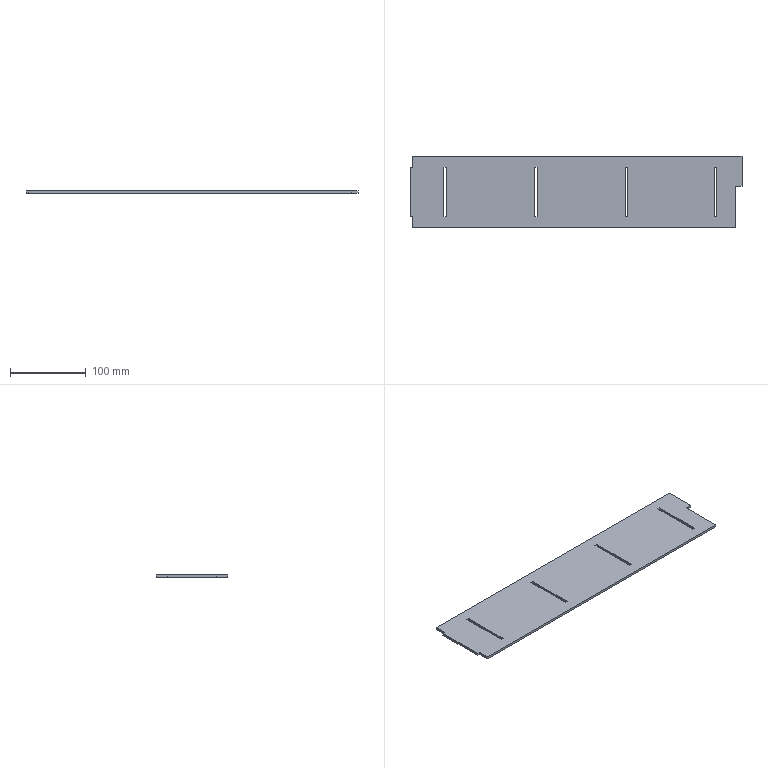Part | SolidWorks | features FlatPattern 1, SMBaseFlange 1, SheetMetal 1 | 1 solid | 28 faces | box 439 x 95 x 3.2 mm | volume 129037 mm3 | plane 28
STEP:
#1=CARTESIAN_POINT('',(218.,0.,3.2));
#2=VERTEX_POINT('',#1);
#3=CARTESIAN_POINT('',(-218.,0.,3.2));
#4=VERTEX_POINT('',#3);
#5=CARTESIAN_POINT('',(218.,0.,3.2));
#6=DIRECTION('',(-1.,0.,0.));
#7=VECTOR('',#6,1000.);
#8=LINE('',#5,#7);
#9=EDGE_CURVE('',#2,#4,#8,.T.);
#10=ORIENTED_EDGE('',*,*,#9,.T.);
#11=CARTESIAN_POINT('',(-218.,-15.,3.2));
#12=VERTEX_POINT('',#11);
#13=CARTESIAN_POINT('',(-218.,0.,3.2));
#14=DIRECTION('',(0.,-1.,0.));
#15=VECTOR('',#14,1000.);
#16=LINE('',#13,#15);
#17=EDGE_CURVE('',#4,#12,#16,.T.);
#18=ORIENTED_EDGE('',*,*,#17,.T.);
#19=CARTESIAN_POINT('',(-221.,-15.,3.2));
#20=VERTEX_POINT('',#19);
#21=CARTESIAN_POINT('',(-218.,-15.,3.2));
#22=DIRECTION('',(-1.,0.,0.));
#23=VECTOR('',#22,1000.);
#24=LINE('',#21,#23);
#25=EDGE_CURVE('',#12,#20,#24,.T.);
#26=ORIENTED_EDGE('',*,*,#25,.T.);
#27=CARTESIAN_POINT('',(-221.,-80.,3.2));
#28=VERTEX_POINT('',#27);
#29=CARTESIAN_POINT('',(-221.,-15.,3.2));
#30=DIRECTION('',(0.,-1.,0.));
#31=VECTOR('',#30,1000.);
#32=LINE('',#29,#31);
#33=EDGE_CURVE('',#20,#28,#32,.T.);
#34=ORIENTED_EDGE('',*,*,#33,.T.);
#35=CARTESIAN_POINT('',(-218.,-80.,3.2));
#36=VERTEX_POINT('',#35);
#37=CARTESIAN_POINT('',(-221.,-80.,3.2));
#38=DIRECTION('',(1.,0.,0.));
#39=VECTOR('',#38,1000.);
#40=LINE('',#37,#39);
#41=EDGE_CURVE('',#28,#36,#40,.T.);
#42=ORIENTED_EDGE('',*,*,#41,.T.);
#43=CARTESIAN_POINT('',(-218.,-95.,3.2));
#44=VERTEX_POINT('',#43);
#45=CARTESIAN_POINT('',(-218.,-80.,3.2));
#46=DIRECTION('',(0.,-1.,0.));
#47=VECTOR('',#46,1000.);
#48=LINE('',#45,#47);
#49=EDGE_CURVE('',#36,#44,#48,.T.);
#50=ORIENTED_EDGE('',*,*,#49,.T.);
#51=CARTESIAN_POINT('',(209.7,-95.,3.2));
#52=VERTEX_POINT('',#51);
#53=CARTESIAN_POINT('',(-218.,-95.,3.2));
#54=DIRECTION('',(1.,0.,0.));
#55=VECTOR('',#54,1000.);
#56=LINE('',#53,#55);
#57=EDGE_CURVE('',#44,#52,#56,.T.);
#58=ORIENTED_EDGE('',*,*,#57,.T.);
#59=CARTESIAN_POINT('',(209.7,-39.7,3.2));
#60=VERTEX_POINT('',#59);
#61=CARTESIAN_POINT('',(209.7,-95.,3.2));
#62=DIRECTION('',(0.,1.,0.));
#63=VECTOR('',#62,1000.);
#64=LINE('',#61,#63);
#65=EDGE_CURVE('',#52,#60,#64,.T.);
#66=ORIENTED_EDGE('',*,*,#65,.T.);
#67=CARTESIAN_POINT('',(218.,-39.7,3.2));
#68=VERTEX_POINT('',#67);
#69=CARTESIAN_POINT('',(209.7,-39.7,3.2));
#70=DIRECTION('',(1.,0.,0.));
#71=VECTOR('',#70,1000.);
#72=LINE('',#69,#71);
#73=EDGE_CURVE('',#60,#68,#72,.T.);
#74=ORIENTED_EDGE('',*,*,#73,.T.);
#75=CARTESIAN_POINT('',(218.,-39.7,3.2));
#76=DIRECTION('',(0.,1.,0.));
#77=VECTOR('',#76,1000.);
#78=LINE('',#75,#77);
#79=EDGE_CURVE('',#68,#2,#78,.T.);
#80=ORIENTED_EDGE('',*,*,#79,.T.);
#81=EDGE_LOOP('',(#10,#18,#26,#34,#42,#50,#58,#66,#74,#80));
#82=FACE_OUTER_BOUND('',#81,.T.);
#83=CARTESIAN_POINT('',(181.5,-80.,3.2));
#84=VERTEX_POINT('',#83);
#85=CARTESIAN_POINT('',(184.7,-80.,3.2));
#86=VERTEX_POINT('',#85);
#87=CARTESIAN_POINT('',(181.5,-80.,3.2));
#88=DIRECTION('',(1.,0.,0.));
#89=VECTOR('',#88,1000.);
#90=LINE('',#87,#89);
#91=EDGE_CURVE('',#84,#86,#90,.T.);
#92=ORIENTED_EDGE('',*,*,#91,.F.);
#93=CARTESIAN_POINT('',(181.5,-15.,3.2));
#94=VERTEX_POINT('',#93);
#95=CARTESIAN_POINT('',(181.5,-15.,3.2));
#96=DIRECTION('',(0.,-1.,0.));
#97=VECTOR('',#96,1000.);
#98=LINE('',#95,#97);
#99=EDGE_CURVE('',#94,#84,#98,.T.);
#100=ORIENTED_EDGE('',*,*,#99,.F.);
#101=CARTESIAN_POINT('',(184.7,-15.,3.2));
#102=VERTEX_POINT('',#101);
#103=CARTESIAN_POINT('',(181.5,-15.,3.2));
#104=DIRECTION('',(-1.,0.,0.));
#105=VECTOR('',#104,1000.);
#106=LINE('',#103,#105);
#107=EDGE_CURVE('',#102,#94,#106,.T.);
#108=ORIENTED_EDGE('',*,*,#107,.F.);
#109=CARTESIAN_POINT('',(184.7,-15.,3.2));
#110=DIRECTION('',(0.,1.,0.));
#111=VECTOR('',#110,1000.);
#112=LINE('',#109,#111);
#113=EDGE_CURVE('',#86,#102,#112,.T.);
#114=ORIENTED_EDGE('',*,*,#113,.F.);
#115=EDGE_LOOP('',(#92,#100,#108,#114));
#116=FACE_BOUND('',#115,.T.);
#117=CARTESIAN_POINT('',(63.8,-80.,3.2));
#118=VERTEX_POINT('',#117);
#119=CARTESIAN_POINT('',(67.,-80.,3.2));
#120=VERTEX_POINT('',#119);
#121=CARTESIAN_POINT('',(63.8,-80.,3.2));
#122=DIRECTION('',(1.,0.,0.));
#123=VECTOR('',#122,1000.);
#124=LINE('',#121,#123);
#125=EDGE_CURVE('',#118,#120,#124,.T.);
#126=ORIENTED_EDGE('',*,*,#125,.F.);
#127=CARTESIAN_POINT('',(63.8,-15.,3.2));
#128=VERTEX_POINT('',#127);
#129=CARTESIAN_POINT('',(63.8,-15.,3.2));
#130=DIRECTION('',(0.,-1.,0.));
#131=VECTOR('',#130,1000.);
#132=LINE('',#129,#131);
#133=EDGE_CURVE('',#128,#118,#132,.T.);
#134=ORIENTED_EDGE('',*,*,#133,.F.);
#135=CARTESIAN_POINT('',(67.,-15.,3.2));
#136=VERTEX_POINT('',#135);
#137=CARTESIAN_POINT('',(63.8,-15.,3.2));
#138=DIRECTION('',(-1.,0.,0.));
#139=VECTOR('',#138,1000.);
#140=LINE('',#137,#139);
#141=EDGE_CURVE('',#136,#128,#140,.T.);
#142=ORIENTED_EDGE('',*,*,#141,.F.);
#143=CARTESIAN_POINT('',(67.,-15.,3.2));
#144=DIRECTION('',(0.,1.,0.));
#145=VECTOR('',#144,1000.);
#146=LINE('',#143,#145);
#147=EDGE_CURVE('',#120,#136,#146,.T.);
#148=ORIENTED_EDGE('',*,*,#147,.F.);
#149=EDGE_LOOP('',(#126,#134,#142,#148));
#150=FACE_BOUND('',#149,.T.);
#151=CARTESIAN_POINT('',(-56.2,-80.,3.2));
#152=VERTEX_POINT('',#151);
#153=CARTESIAN_POINT('',(-53.,-80.,3.2));
#154=VERTEX_POINT('',#153);
#155=CARTESIAN_POINT('',(-56.2,-80.,3.2));
#156=DIRECTION('',(1.,0.,0.));
#157=VECTOR('',#156,1000.);
#158=LINE('',#155,#157);
#159=EDGE_CURVE('',#152,#154,#158,.T.);
#160=ORIENTED_EDGE('',*,*,#159,.F.);
#161=CARTESIAN_POINT('',(-56.2,-15.,3.2));
#162=VERTEX_POINT('',#161);
#163=CARTESIAN_POINT('',(-56.2,-15.,3.2));
#164=DIRECTION('',(0.,-1.,0.));
#165=VECTOR('',#164,1000.);
#166=LINE('',#163,#165);
#167=EDGE_CURVE('',#162,#152,#166,.T.);
#168=ORIENTED_EDGE('',*,*,#167,.F.);
#169=CARTESIAN_POINT('',(-53.,-15.,3.2));
#170=VERTEX_POINT('',#169);
#171=CARTESIAN_POINT('',(-56.2,-15.,3.2));
#172=DIRECTION('',(-1.,0.,0.));
#173=VECTOR('',#172,1000.);
#174=LINE('',#171,#173);
#175=EDGE_CURVE('',#170,#162,#174,.T.);
#176=ORIENTED_EDGE('',*,*,#175,.F.);
#177=CARTESIAN_POINT('',(-53.,-15.,3.2));
#178=DIRECTION('',(0.,1.,0.));
#179=VECTOR('',#178,1000.);
#180=LINE('',#177,#179);
#181=EDGE_CURVE('',#154,#170,#180,.T.);
#182=ORIENTED_EDGE('',*,*,#181,.F.);
#183=EDGE_LOOP('',(#160,#168,#176,#182));
#184=FACE_BOUND('',#183,.T.);
#185=CARTESIAN_POINT('',(-176.2,-80.,3.2));
#186=VERTEX_POINT('',#185);
#187=CARTESIAN_POINT('',(-173.,-80.,3.2));
#188=VERTEX_POINT('',#187);
#189=CARTESIAN_POINT('',(-176.2,-80.,3.2));
#190=DIRECTION('',(1.,0.,0.));
#191=VECTOR('',#190,1000.);
#192=LINE('',#189,#191);
#193=EDGE_CURVE('',#186,#188,#192,.T.);
#194=ORIENTED_EDGE('',*,*,#193,.F.);
#195=CARTESIAN_POINT('',(-176.2,-15.,3.2));
#196=VERTEX_POINT('',#195);
#197=CARTESIAN_POINT('',(-176.2,-15.,3.2));
#198=DIRECTION('',(0.,-1.,0.));
#199=VECTOR('',#198,1000.);
#200=LINE('',#197,#199);
#201=EDGE_CURVE('',#196,#186,#200,.T.);
#202=ORIENTED_EDGE('',*,*,#201,.F.);
#203=CARTESIAN_POINT('',(-173.,-15.,3.2));
#204=VERTEX_POINT('',#203);
#205=CARTESIAN_POINT('',(-176.2,-15.,3.2));
#206=DIRECTION('',(-1.,0.,0.));
#207=VECTOR('',#206,1000.);
#208=LINE('',#205,#207);
#209=EDGE_CURVE('',#204,#196,#208,.T.);
#210=ORIENTED_EDGE('',*,*,#209,.F.);
#211=CARTESIAN_POINT('',(-173.,-15.,3.2));
#212=DIRECTION('',(0.,1.,0.));
#213=VECTOR('',#212,1000.);
#214=LINE('',#211,#213);
#215=EDGE_CURVE('',#188,#204,#214,.T.);
#216=ORIENTED_EDGE('',*,*,#215,.F.);
#217=EDGE_LOOP('',(#194,#202,#210,#216));
#218=FACE_BOUND('',#217,.T.);
#219=CARTESIAN_POINT('',(0.,0.,3.2));
#220=DIRECTION('',(0.,0.,1.));
#221=DIRECTION('',(1.,0.,0.));
#222=AXIS2_PLACEMENT_3D('',#219,#220,#221);
#223=PLANE('',#222);
#224=ADVANCED_FACE('',(#82,#116,#150,#184,#218),#223,.T.);
#225=CARTESIAN_POINT('',(-56.2,-15.,0.));
#226=VERTEX_POINT('',#225);
#227=CARTESIAN_POINT('',(-56.2,-80.,0.));
#228=VERTEX_POINT('',#227);
#229=CARTESIAN_POINT('',(-56.2,-15.,0.));
#230=DIRECTION('',(0.,-1.,0.));
#231=VECTOR('',#230,1000.);
#232=LINE('',#229,#231);
#233=EDGE_CURVE('',#226,#228,#232,.T.);
#234=ORIENTED_EDGE('',*,*,#233,.T.);
#235=CARTESIAN_POINT('',(-53.,-80.,0.));
#236=VERTEX_POINT('',#235);
#237=CARTESIAN_POINT('',(-56.2,-80.,0.));
#238=DIRECTION('',(1.,0.,0.));
#239=VECTOR('',#238,1000.);
#240=LINE('',#237,#239);
#241=EDGE_CURVE('',#228,#236,#240,.T.);
#242=ORIENTED_EDGE('',*,*,#241,.T.);
#243=CARTESIAN_POINT('',(-53.,-15.,0.));
#244=VERTEX_POINT('',#243);
#245=CARTESIAN_POINT('',(-53.,-15.,0.));
#246=DIRECTION('',(0.,1.,0.));
#247=VECTOR('',#246,1000.);
#248=LINE('',#245,#247);
#249=EDGE_CURVE('',#236,#244,#248,.T.);
#250=ORIENTED_EDGE('',*,*,#249,.T.);
#251=CARTESIAN_POINT('',(-56.2,-15.,0.));
#252=DIRECTION('',(-1.,0.,0.));
#253=VECTOR('',#252,1000.);
#254=LINE('',#251,#253);
#255=EDGE_CURVE('',#244,#226,#254,.T.);
#256=ORIENTED_EDGE('',*,*,#255,.T.);
#257=EDGE_LOOP('',(#234,#242,#250,#256));
#258=FACE_BOUND('',#257,.T.);
#259=CARTESIAN_POINT('',(181.5,-15.,0.));
#260=VERTEX_POINT('',#259);
#261=CARTESIAN_POINT('',(181.5,-80.,0.));
#262=VERTEX_POINT('',#261);
#263=CARTESIAN_POINT('',(181.5,-15.,0.));
#264=DIRECTION('',(0.,-1.,0.));
#265=VECTOR('',#264,1000.);
#266=LINE('',#263,#265);
#267=EDGE_CURVE('',#260,#262,#266,.T.);
#268=ORIENTED_EDGE('',*,*,#267,.T.);
#269=CARTESIAN_POINT('',(184.7,-80.,0.));
#270=VERTEX_POINT('',#269);
#271=CARTESIAN_POINT('',(181.5,-80.,0.));
#272=DIRECTION('',(1.,0.,0.));
#273=VECTOR('',#272,1000.);
#274=LINE('',#271,#273);
#275=EDGE_CURVE('',#262,#270,#274,.T.);
#276=ORIENTED_EDGE('',*,*,#275,.T.);
#277=CARTESIAN_POINT('',(184.7,-15.,0.));
#278=VERTEX_POINT('',#277);
#279=CARTESIAN_POINT('',(184.7,-15.,0.));
#280=DIRECTION('',(0.,1.,0.));
#281=VECTOR('',#280,1000.);
#282=LINE('',#279,#281);
#283=EDGE_CURVE('',#270,#278,#282,.T.);
#284=ORIENTED_EDGE('',*,*,#283,.T.);
#285=CARTESIAN_POINT('',(181.5,-15.,0.));
#286=DIRECTION('',(-1.,0.,0.));
#287=VECTOR('',#286,1000.);
#288=LINE('',#285,#287);
#289=EDGE_CURVE('',#278,#260,#288,.T.);
#290=ORIENTED_EDGE('',*,*,#289,.T.);
#291=EDGE_LOOP('',(#268,#276,#284,#290));
#292=FACE_BOUND('',#291,.T.);
#293=CARTESIAN_POINT('',(218.,0.,0.));
#294=VERTEX_POINT('',#293);
#295=CARTESIAN_POINT('',(-218.,0.,0.));
#296=VERTEX_POINT('',#295);
#297=CARTESIAN_POINT('',(218.,0.,0.));
#298=DIRECTION('',(-1.,0.,0.));
#299=VECTOR('',#298,1000.);
#300=LINE('',#297,#299);
#301=EDGE_CURVE('',#294,#296,#300,.T.);
#302=ORIENTED_EDGE('',*,*,#301,.F.);
#303=CARTESIAN_POINT('',(218.,-39.7,0.));
#304=VERTEX_POINT('',#303);
#305=CARTESIAN_POINT('',(218.,-39.7,0.));
#306=DIRECTION('',(0.,1.,0.));
#307=VECTOR('',#306,1000.);
#308=LINE('',#305,#307);
#309=EDGE_CURVE('',#304,#294,#308,.T.);
#310=ORIENTED_EDGE('',*,*,#309,.F.);
#311=CARTESIAN_POINT('',(209.7,-39.7,0.));
#312=VERTEX_POINT('',#311);
#313=CARTESIAN_POINT('',(209.7,-39.7,0.));
#314=DIRECTION('',(1.,0.,0.));
#315=VECTOR('',#314,1000.);
#316=LINE('',#313,#315);
#317=EDGE_CURVE('',#312,#304,#316,.T.);
#318=ORIENTED_EDGE('',*,*,#317,.F.);
#319=CARTESIAN_POINT('',(209.7,-95.,0.));
#320=VERTEX_POINT('',#319);
#321=CARTESIAN_POINT('',(209.7,-95.,0.));
#322=DIRECTION('',(0.,1.,0.));
#323=VECTOR('',#322,1000.);
#324=LINE('',#321,#323);
#325=EDGE_CURVE('',#320,#312,#324,.T.);
#326=ORIENTED_EDGE('',*,*,#325,.F.);
#327=CARTESIAN_POINT('',(-218.,-95.,0.));
#328=VERTEX_POINT('',#327);
#329=CARTESIAN_POINT('',(-218.,-95.,0.));
#330=DIRECTION('',(1.,0.,0.));
#331=VECTOR('',#330,1000.);
#332=LINE('',#329,#331);
#333=EDGE_CURVE('',#328,#320,#332,.T.);
#334=ORIENTED_EDGE('',*,*,#333,.F.);
#335=CARTESIAN_POINT('',(-218.,-80.,0.));
#336=VERTEX_POINT('',#335);
#337=CARTESIAN_POINT('',(-218.,-80.,0.));
#338=DIRECTION('',(0.,-1.,0.));
#339=VECTOR('',#338,1000.);
#340=LINE('',#337,#339);
#341=EDGE_CURVE('',#336,#328,#340,.T.);
#342=ORIENTED_EDGE('',*,*,#341,.F.);
#343=CARTESIAN_POINT('',(-221.,-80.,0.));
#344=VERTEX_POINT('',#343);
#345=CARTESIAN_POINT('',(-221.,-80.,0.));
#346=DIRECTION('',(1.,0.,0.));
#347=VECTOR('',#346,1000.);
#348=LINE('',#345,#347);
#349=EDGE_CURVE('',#344,#336,#348,.T.);
#350=ORIENTED_EDGE('',*,*,#349,.F.);
#351=CARTESIAN_POINT('',(-221.,-15.,0.));
#352=VERTEX_POINT('',#351);
#353=CARTESIAN_POINT('',(-221.,-15.,0.));
#354=DIRECTION('',(0.,-1.,0.));
#355=VECTOR('',#354,1000.);
#356=LINE('',#353,#355);
#357=EDGE_CURVE('',#352,#344,#356,.T.);
#358=ORIENTED_EDGE('',*,*,#357,.F.);
#359=CARTESIAN_POINT('',(-218.,-15.,0.));
#360=VERTEX_POINT('',#359);
#361=CARTESIAN_POINT('',(-218.,-15.,0.));
#362=DIRECTION('',(-1.,0.,0.));
#363=VECTOR('',#362,1000.);
#364=LINE('',#361,#363);
#365=EDGE_CURVE('',#360,#352,#364,.T.);
#366=ORIENTED_EDGE('',*,*,#365,.F.);
#367=CARTESIAN_POINT('',(-218.,0.,0.));
#368=DIRECTION('',(0.,-1.,0.));
#369=VECTOR('',#368,1000.);
#370=LINE('',#367,#369);
#371=EDGE_CURVE('',#296,#360,#370,.T.);
#372=ORIENTED_EDGE('',*,*,#371,.F.);
#373=EDGE_LOOP('',(#302,#310,#318,#326,#334,#342,#350,#358,#366,#372));
#374=FACE_OUTER_BOUND('',#373,.T.);
#375=CARTESIAN_POINT('',(63.8,-15.,0.));
#376=VERTEX_POINT('',#375);
#377=CARTESIAN_POINT('',(63.8,-80.,0.));
#378=VERTEX_POINT('',#377);
#379=CARTESIAN_POINT('',(63.8,-15.,0.));
#380=DIRECTION('',(0.,-1.,0.));
#381=VECTOR('',#380,1000.);
#382=LINE('',#379,#381);
#383=EDGE_CURVE('',#376,#378,#382,.T.);
#384=ORIENTED_EDGE('',*,*,#383,.T.);
#385=CARTESIAN_POINT('',(67.,-80.,0.));
#386=VERTEX_POINT('',#385);
#387=CARTESIAN_POINT('',(63.8,-80.,0.));
#388=DIRECTION('',(1.,0.,0.));
#389=VECTOR('',#388,1000.);
#390=LINE('',#387,#389);
#391=EDGE_CURVE('',#378,#386,#390,.T.);
#392=ORIENTED_EDGE('',*,*,#391,.T.);
#393=CARTESIAN_POINT('',(67.,-15.,0.));
#394=VERTEX_POINT('',#393);
#395=CARTESIAN_POINT('',(67.,-15.,0.));
#396=DIRECTION('',(0.,1.,0.));
#397=VECTOR('',#396,1000.);
#398=LINE('',#395,#397);
#399=EDGE_CURVE('',#386,#394,#398,.T.);
#400=ORIENTED_EDGE('',*,*,#399,.T.);
#401=CARTESIAN_POINT('',(63.8,-15.,0.));
#402=DIRECTION('',(-1.,0.,0.));
#403=VECTOR('',#402,1000.);
#404=LINE('',#401,#403);
#405=EDGE_CURVE('',#394,#376,#404,.T.);
#406=ORIENTED_EDGE('',*,*,#405,.T.);
#407=EDGE_LOOP('',(#384,#392,#400,#406));
#408=FACE_BOUND('',#407,.T.);
#409=CARTESIAN_POINT('',(-176.2,-15.,0.));
#410=VERTEX_POINT('',#409);
#411=CARTESIAN_POINT('',(-176.2,-80.,0.));
#412=VERTEX_POINT('',#411);
#413=CARTESIAN_POINT('',(-176.2,-15.,0.));
#414=DIRECTION('',(0.,-1.,0.));
#415=VECTOR('',#414,1000.);
#416=LINE('',#413,#415);
#417=EDGE_CURVE('',#410,#412,#416,.T.);
#418=ORIENTED_EDGE('',*,*,#417,.T.);
#419=CARTESIAN_POINT('',(-173.,-80.,0.));
#420=VERTEX_POINT('',#419);
#421=CARTESIAN_POINT('',(-176.2,-80.,0.));
#422=DIRECTION('',(1.,0.,0.));
#423=VECTOR('',#422,1000.);
#424=LINE('',#421,#423);
#425=EDGE_CURVE('',#412,#420,#424,.T.);
#426=ORIENTED_EDGE('',*,*,#425,.T.);
#427=CARTESIAN_POINT('',(-173.,-15.,0.));
#428=VERTEX_POINT('',#427);
#429=CARTESIAN_POINT('',(-173.,-15.,0.));
#430=DIRECTION('',(0.,1.,0.));
#431=VECTOR('',#430,1000.);
#432=LINE('',#429,#431);
#433=EDGE_CURVE('',#420,#428,#432,.T.);
#434=ORIENTED_EDGE('',*,*,#433,.T.);
#435=CARTESIAN_POINT('',(-176.2,-15.,0.));
#436=DIRECTION('',(-1.,0.,0.));
#437=VECTOR('',#436,1000.);
#438=LINE('',#435,#437);
#439=EDGE_CURVE('',#428,#410,#438,.T.);
#440=ORIENTED_EDGE('',*,*,#439,.T.);
#441=EDGE_LOOP('',(#418,#426,#434,#440));
#442=FACE_BOUND('',#441,.T.);
#443=CARTESIAN_POINT('',(0.,0.,0.));
#444=DIRECTION('',(0.,0.,1.));
#445=DIRECTION('',(1.,0.,0.));
#446=AXIS2_PLACEMENT_3D('',#443,#444,#445);
#447=PLANE('',#446);
#448=ADVANCED_FACE('',(#258,#292,#374,#408,#442),#447,.F.);
#449=ORIENTED_EDGE('',*,*,#301,.T.);
#450=CARTESIAN_POINT('',(-218.,0.,3.2));
#451=DIRECTION('',(0.,0.,-1.));
#452=VECTOR('',#451,1000.);
#453=LINE('',#450,#452);
#454=EDGE_CURVE('',#4,#296,#453,.T.);
#455=ORIENTED_EDGE('',*,*,#454,.F.);
#456=ORIENTED_EDGE('',*,*,#9,.F.);
#457=CARTESIAN_POINT('',(218.,0.,3.2));
#458=DIRECTION('',(0.,0.,-1.));
#459=VECTOR('',#458,1000.);
#460=LINE('',#457,#459);
#461=EDGE_CURVE('',#2,#294,#460,.T.);
#462=ORIENTED_EDGE('',*,*,#461,.T.);
#463=EDGE_LOOP('',(#449,#455,#456,#462));
#464=FACE_OUTER_BOUND('',#463,.T.);
#465=CARTESIAN_POINT('',(218.,0.,3.2));
#466=DIRECTION('',(0.,-1.,0.));
#467=DIRECTION('',(1.,0.,0.));
#468=AXIS2_PLACEMENT_3D('',#465,#466,#467);
#469=PLANE('',#468);
#470=ADVANCED_FACE('',(#464),#469,.F.);
#471=ORIENTED_EDGE('',*,*,#371,.T.);
#472=CARTESIAN_POINT('',(-218.,-15.,3.2));
#473=DIRECTION('',(0.,0.,-1.));
#474=VECTOR('',#473,1000.);
#475=LINE('',#472,#474);
#476=EDGE_CURVE('',#12,#360,#475,.T.);
#477=ORIENTED_EDGE('',*,*,#476,.F.);
#478=ORIENTED_EDGE('',*,*,#17,.F.);
#479=ORIENTED_EDGE('',*,*,#454,.T.);
#480=EDGE_LOOP('',(#471,#477,#478,#479));
#481=FACE_OUTER_BOUND('',#480,.T.);
#482=CARTESIAN_POINT('',(-218.,0.,3.2));
#483=DIRECTION('',(1.,0.,0.));
#484=DIRECTION('',(0.,0.,-1.));
#485=AXIS2_PLACEMENT_3D('',#482,#483,#484);
#486=PLANE('',#485);
#487=ADVANCED_FACE('',(#481),#486,.F.);
#488=ORIENTED_EDGE('',*,*,#365,.T.);
#489=CARTESIAN_POINT('',(-221.,-15.,3.2));
#490=DIRECTION('',(0.,0.,-1.));
#491=VECTOR('',#490,1000.);
#492=LINE('',#489,#491);
#493=EDGE_CURVE('',#20,#352,#492,.T.);
#494=ORIENTED_EDGE('',*,*,#493,.F.);
#495=ORIENTED_EDGE('',*,*,#25,.F.);
#496=ORIENTED_EDGE('',*,*,#476,.T.);
#497=EDGE_LOOP('',(#488,#494,#495,#496));
#498=FACE_OUTER_BOUND('',#497,.T.);
#499=CARTESIAN_POINT('',(-218.,-15.,3.2));
#500=DIRECTION('',(0.,-1.,0.));
#501=DIRECTION('',(0.,0.,-1.));
#502=AXIS2_PLACEMENT_3D('',#499,#500,#501);
#503=PLANE('',#502);
#504=ADVANCED_FACE('',(#498),#503,.F.);
#505=ORIENTED_EDGE('',*,*,#357,.T.);
#506=CARTESIAN_POINT('',(-221.,-80.,3.2));
#507=DIRECTION('',(0.,0.,-1.));
#508=VECTOR('',#507,1000.);
#509=LINE('',#506,#508);
#510=EDGE_CURVE('',#28,#344,#509,.T.);
#511=ORIENTED_EDGE('',*,*,#510,.F.);
#512=ORIENTED_EDGE('',*,*,#33,.F.);
#513=ORIENTED_EDGE('',*,*,#493,.T.);
#514=EDGE_LOOP('',(#505,#511,#512,#513));
#515=FACE_OUTER_BOUND('',#514,.T.);
#516=CARTESIAN_POINT('',(-221.,-15.,3.2));
#517=DIRECTION('',(1.,0.,0.));
#518=DIRECTION('',(0.,1.,0.));
#519=AXIS2_PLACEMENT_3D('',#516,#517,#518);
#520=PLANE('',#519);
#521=ADVANCED_FACE('',(#515),#520,.F.);
#522=ORIENTED_EDGE('',*,*,#349,.T.);
#523=CARTESIAN_POINT('',(-218.,-80.,3.2));
#524=DIRECTION('',(0.,0.,-1.));
#525=VECTOR('',#524,1000.);
#526=LINE('',#523,#525);
#527=EDGE_CURVE('',#36,#336,#526,.T.);
#528=ORIENTED_EDGE('',*,*,#527,.F.);
#529=ORIENTED_EDGE('',*,*,#41,.F.);
#530=ORIENTED_EDGE('',*,*,#510,.T.);
#531=EDGE_LOOP('',(#522,#528,#529,#530));
#532=FACE_OUTER_BOUND('',#531,.T.);
#533=CARTESIAN_POINT('',(-221.,-80.,3.2));
#534=DIRECTION('',(0.,1.,0.));
#535=DIRECTION('',(0.,0.,1.));
#536=AXIS2_PLACEMENT_3D('',#533,#534,#535);
#537=PLANE('',#536);
#538=ADVANCED_FACE('',(#532),#537,.F.);
#539=ORIENTED_EDGE('',*,*,#341,.T.);
#540=CARTESIAN_POINT('',(-218.,-95.,3.2));
#541=DIRECTION('',(0.,0.,-1.));
#542=VECTOR('',#541,1000.);
#543=LINE('',#540,#542);
#544=EDGE_CURVE('',#44,#328,#543,.T.);
#545=ORIENTED_EDGE('',*,*,#544,.F.);
#546=ORIENTED_EDGE('',*,*,#49,.F.);
#547=ORIENTED_EDGE('',*,*,#527,.T.);
#548=EDGE_LOOP('',(#539,#545,#546,#547));
#549=FACE_OUTER_BOUND('',#548,.T.);
#550=CARTESIAN_POINT('',(-218.,-80.,3.2));
#551=DIRECTION('',(1.,0.,0.));
#552=DIRECTION('',(0.,0.,-1.));
#553=AXIS2_PLACEMENT_3D('',#550,#551,#552);
#554=PLANE('',#553);
#555=ADVANCED_FACE('',(#549),#554,.F.);
#556=ORIENTED_EDGE('',*,*,#333,.T.);
#557=CARTESIAN_POINT('',(209.7,-95.,3.2));
#558=DIRECTION('',(0.,0.,-1.));
#559=VECTOR('',#558,1000.);
#560=LINE('',#557,#559);
#561=EDGE_CURVE('',#52,#320,#560,.T.);
#562=ORIENTED_EDGE('',*,*,#561,.F.);
#563=ORIENTED_EDGE('',*,*,#57,.F.);
#564=ORIENTED_EDGE('',*,*,#544,.T.);
#565=EDGE_LOOP('',(#556,#562,#563,#564));
#566=FACE_OUTER_BOUND('',#565,.T.);
#567=CARTESIAN_POINT('',(-218.,-95.,3.2));
#568=DIRECTION('',(0.,1.,0.));
#569=DIRECTION('',(0.,0.,1.));
#570=AXIS2_PLACEMENT_3D('',#567,#568,#569);
#571=PLANE('',#570);
#572=ADVANCED_FACE('',(#566),#571,.F.);
#573=ORIENTED_EDGE('',*,*,#325,.T.);
#574=CARTESIAN_POINT('',(209.7,-39.7,3.2));
#575=DIRECTION('',(0.,0.,-1.));
#576=VECTOR('',#575,1000.);
#577=LINE('',#574,#576);
#578=EDGE_CURVE('',#60,#312,#577,.T.);
#579=ORIENTED_EDGE('',*,*,#578,.F.);
#580=ORIENTED_EDGE('',*,*,#65,.F.);
#581=ORIENTED_EDGE('',*,*,#561,.T.);
#582=EDGE_LOOP('',(#573,#579,#580,#581));
#583=FACE_OUTER_BOUND('',#582,.T.);
#584=CARTESIAN_POINT('',(209.7,-95.,3.2));
#585=DIRECTION('',(-1.,0.,0.));
#586=DIRECTION('',(0.,0.,1.));
#587=AXIS2_PLACEMENT_3D('',#584,#585,#586);
#588=PLANE('',#587);
#589=ADVANCED_FACE('',(#583),#588,.F.);
#590=ORIENTED_EDGE('',*,*,#317,.T.);
#591=CARTESIAN_POINT('',(218.,-39.7,3.2));
#592=DIRECTION('',(0.,0.,-1.));
#593=VECTOR('',#592,1000.);
#594=LINE('',#591,#593);
#595=EDGE_CURVE('',#68,#304,#594,.T.);
#596=ORIENTED_EDGE('',*,*,#595,.F.);
#597=ORIENTED_EDGE('',*,*,#73,.F.);
#598=ORIENTED_EDGE('',*,*,#578,.T.);
#599=EDGE_LOOP('',(#590,#596,#597,#598));
#600=FACE_OUTER_BOUND('',#599,.T.);
#601=CARTESIAN_POINT('',(209.7,-39.7,3.2));
#602=DIRECTION('',(0.,1.,0.));
#603=DIRECTION('',(0.,0.,1.));
#604=AXIS2_PLACEMENT_3D('',#601,#602,#603);
#605=PLANE('',#604);
#606=ADVANCED_FACE('',(#600),#605,.F.);
#607=ORIENTED_EDGE('',*,*,#309,.T.);
#608=ORIENTED_EDGE('',*,*,#461,.F.);
#609=ORIENTED_EDGE('',*,*,#79,.F.);
#610=ORIENTED_EDGE('',*,*,#595,.T.);
#611=EDGE_LOOP('',(#607,#608,#609,#610));
#612=FACE_OUTER_BOUND('',#611,.T.);
#613=CARTESIAN_POINT('',(218.,-39.7,3.2));
#614=DIRECTION('',(-1.,0.,0.));
#615=DIRECTION('',(0.,0.,1.));
#616=AXIS2_PLACEMENT_3D('',#613,#614,#615);
#617=PLANE('',#616);
#618=ADVANCED_FACE('',(#612),#617,.F.);
#619=ORIENTED_EDGE('',*,*,#267,.F.);
#620=CARTESIAN_POINT('',(181.5,-15.,3.2));
#621=DIRECTION('',(0.,0.,-1.));
#622=VECTOR('',#621,1000.);
#623=LINE('',#620,#622);
#624=EDGE_CURVE('',#94,#260,#623,.T.);
#625=ORIENTED_EDGE('',*,*,#624,.F.);
#626=ORIENTED_EDGE('',*,*,#99,.T.);
#627=CARTESIAN_POINT('',(181.5,-80.,3.2));
#628=DIRECTION('',(0.,0.,-1.));
#629=VECTOR('',#628,1000.);
#630=LINE('',#627,#629);
#631=EDGE_CURVE('',#84,#262,#630,.T.);
#632=ORIENTED_EDGE('',*,*,#631,.T.);
#633=EDGE_LOOP('',(#619,#625,#626,#632));
#634=FACE_OUTER_BOUND('',#633,.T.);
#635=CARTESIAN_POINT('',(181.5,-15.,3.2));
#636=DIRECTION('',(1.,0.,0.));
#637=DIRECTION('',(0.,0.,-1.));
#638=AXIS2_PLACEMENT_3D('',#635,#636,#637);
#639=PLANE('',#638);
#640=ADVANCED_FACE('',(#634),#639,.T.);
#641=ORIENTED_EDGE('',*,*,#275,.F.);
#642=ORIENTED_EDGE('',*,*,#631,.F.);
#643=ORIENTED_EDGE('',*,*,#91,.T.);
#644=CARTESIAN_POINT('',(184.7,-80.,3.2));
#645=DIRECTION('',(0.,0.,-1.));
#646=VECTOR('',#645,1000.);
#647=LINE('',#644,#646);
#648=EDGE_CURVE('',#86,#270,#647,.T.);
#649=ORIENTED_EDGE('',*,*,#648,.T.);
#650=EDGE_LOOP('',(#641,#642,#643,#649));
#651=FACE_OUTER_BOUND('',#650,.T.);
#652=CARTESIAN_POINT('',(181.5,-80.,3.2));
#653=DIRECTION('',(0.,1.,0.));
#654=DIRECTION('',(0.,0.,1.));
#655=AXIS2_PLACEMENT_3D('',#652,#653,#654);
#656=PLANE('',#655);
#657=ADVANCED_FACE('',(#651),#656,.T.);
#658=ORIENTED_EDGE('',*,*,#283,.F.);
#659=ORIENTED_EDGE('',*,*,#648,.F.);
#660=ORIENTED_EDGE('',*,*,#113,.T.);
#661=CARTESIAN_POINT('',(184.7,-15.,3.2));
#662=DIRECTION('',(0.,0.,-1.));
#663=VECTOR('',#662,1000.);
#664=LINE('',#661,#663);
#665=EDGE_CURVE('',#102,#278,#664,.T.);
#666=ORIENTED_EDGE('',*,*,#665,.T.);
#667=EDGE_LOOP('',(#658,#659,#660,#666));
#668=FACE_OUTER_BOUND('',#667,.T.);
#669=CARTESIAN_POINT('',(184.7,-15.,3.2));
#670=DIRECTION('',(-1.,0.,0.));
#671=DIRECTION('',(0.,0.,1.));
#672=AXIS2_PLACEMENT_3D('',#669,#670,#671);
#673=PLANE('',#672);
#674=ADVANCED_FACE('',(#668),#673,.T.);
#675=ORIENTED_EDGE('',*,*,#289,.F.);
#676=ORIENTED_EDGE('',*,*,#665,.F.);
#677=ORIENTED_EDGE('',*,*,#107,.T.);
#678=ORIENTED_EDGE('',*,*,#624,.T.);
#679=EDGE_LOOP('',(#675,#676,#677,#678));
#680=FACE_OUTER_BOUND('',#679,.T.);
#681=CARTESIAN_POINT('',(181.5,-15.,3.2));
#682=DIRECTION('',(0.,-1.,0.));
#683=DIRECTION('',(0.,0.,-1.));
#684=AXIS2_PLACEMENT_3D('',#681,#682,#683);
#685=PLANE('',#684);
#686=ADVANCED_FACE('',(#680),#685,.T.);
#687=ORIENTED_EDGE('',*,*,#383,.F.);
#688=CARTESIAN_POINT('',(63.8,-15.,3.2));
#689=DIRECTION('',(0.,0.,-1.));
#690=VECTOR('',#689,1000.);
#691=LINE('',#688,#690);
#692=EDGE_CURVE('',#128,#376,#691,.T.);
#693=ORIENTED_EDGE('',*,*,#692,.F.);
#694=ORIENTED_EDGE('',*,*,#133,.T.);
#695=CARTESIAN_POINT('',(63.8,-80.,3.2));
#696=DIRECTION('',(0.,0.,-1.));
#697=VECTOR('',#696,1000.);
#698=LINE('',#695,#697);
#699=EDGE_CURVE('',#118,#378,#698,.T.);
#700=ORIENTED_EDGE('',*,*,#699,.T.);
#701=EDGE_LOOP('',(#687,#693,#694,#700));
#702=FACE_OUTER_BOUND('',#701,.T.);
#703=CARTESIAN_POINT('',(63.8,-15.,3.2));
#704=DIRECTION('',(1.,0.,0.));
#705=DIRECTION('',(0.,0.,-1.));
#706=AXIS2_PLACEMENT_3D('',#703,#704,#705);
#707=PLANE('',#706);
#708=ADVANCED_FACE('',(#702),#707,.T.);
#709=ORIENTED_EDGE('',*,*,#391,.F.);
#710=ORIENTED_EDGE('',*,*,#699,.F.);
#711=ORIENTED_EDGE('',*,*,#125,.T.);
#712=CARTESIAN_POINT('',(67.,-80.,3.2));
#713=DIRECTION('',(0.,0.,-1.));
#714=VECTOR('',#713,1000.);
#715=LINE('',#712,#714);
#716=EDGE_CURVE('',#120,#386,#715,.T.);
#717=ORIENTED_EDGE('',*,*,#716,.T.);
#718=EDGE_LOOP('',(#709,#710,#711,#717));
#719=FACE_OUTER_BOUND('',#718,.T.);
#720=CARTESIAN_POINT('',(63.8,-80.,3.2));
#721=DIRECTION('',(0.,1.,0.));
#722=DIRECTION('',(0.,0.,1.));
#723=AXIS2_PLACEMENT_3D('',#720,#721,#722);
#724=PLANE('',#723);
#725=ADVANCED_FACE('',(#719),#724,.T.);
#726=ORIENTED_EDGE('',*,*,#399,.F.);
#727=ORIENTED_EDGE('',*,*,#716,.F.);
#728=ORIENTED_EDGE('',*,*,#147,.T.);
#729=CARTESIAN_POINT('',(67.,-15.,3.2));
#730=DIRECTION('',(0.,0.,-1.));
#731=VECTOR('',#730,1000.);
#732=LINE('',#729,#731);
#733=EDGE_CURVE('',#136,#394,#732,.T.);
#734=ORIENTED_EDGE('',*,*,#733,.T.);
#735=EDGE_LOOP('',(#726,#727,#728,#734));
#736=FACE_OUTER_BOUND('',#735,.T.);
#737=CARTESIAN_POINT('',(67.,-15.,3.2));
#738=DIRECTION('',(-1.,0.,0.));
#739=DIRECTION('',(0.,0.,1.));
#740=AXIS2_PLACEMENT_3D('',#737,#738,#739);
#741=PLANE('',#740);
#742=ADVANCED_FACE('',(#736),#741,.T.);
#743=ORIENTED_EDGE('',*,*,#405,.F.);
#744=ORIENTED_EDGE('',*,*,#733,.F.);
#745=ORIENTED_EDGE('',*,*,#141,.T.);
#746=ORIENTED_EDGE('',*,*,#692,.T.);
#747=EDGE_LOOP('',(#743,#744,#745,#746));
#748=FACE_OUTER_BOUND('',#747,.T.);
#749=CARTESIAN_POINT('',(63.8,-15.,3.2));
#750=DIRECTION('',(0.,-1.,0.));
#751=DIRECTION('',(0.,0.,-1.));
#752=AXIS2_PLACEMENT_3D('',#749,#750,#751);
#753=PLANE('',#752);
#754=ADVANCED_FACE('',(#748),#753,.T.);
#755=ORIENTED_EDGE('',*,*,#233,.F.);
#756=CARTESIAN_POINT('',(-56.2,-15.,3.2));
#757=DIRECTION('',(0.,0.,-1.));
#758=VECTOR('',#757,1000.);
#759=LINE('',#756,#758);
#760=EDGE_CURVE('',#162,#226,#759,.T.);
#761=ORIENTED_EDGE('',*,*,#760,.F.);
#762=ORIENTED_EDGE('',*,*,#167,.T.);
#763=CARTESIAN_POINT('',(-56.2,-80.,3.2));
#764=DIRECTION('',(0.,0.,-1.));
#765=VECTOR('',#764,1000.);
#766=LINE('',#763,#765);
#767=EDGE_CURVE('',#152,#228,#766,.T.);
#768=ORIENTED_EDGE('',*,*,#767,.T.);
#769=EDGE_LOOP('',(#755,#761,#762,#768));
#770=FACE_OUTER_BOUND('',#769,.T.);
#771=CARTESIAN_POINT('',(-56.2,-15.,3.2));
#772=DIRECTION('',(1.,0.,0.));
#773=DIRECTION('',(0.,0.,-1.));
#774=AXIS2_PLACEMENT_3D('',#771,#772,#773);
#775=PLANE('',#774);
#776=ADVANCED_FACE('',(#770),#775,.T.);
#777=ORIENTED_EDGE('',*,*,#241,.F.);
#778=ORIENTED_EDGE('',*,*,#767,.F.);
#779=ORIENTED_EDGE('',*,*,#159,.T.);
#780=CARTESIAN_POINT('',(-53.,-80.,3.2));
#781=DIRECTION('',(0.,0.,-1.));
#782=VECTOR('',#781,1000.);
#783=LINE('',#780,#782);
#784=EDGE_CURVE('',#154,#236,#783,.T.);
#785=ORIENTED_EDGE('',*,*,#784,.T.);
#786=EDGE_LOOP('',(#777,#778,#779,#785));
#787=FACE_OUTER_BOUND('',#786,.T.);
#788=CARTESIAN_POINT('',(-56.2,-80.,3.2));
#789=DIRECTION('',(0.,1.,0.));
#790=DIRECTION('',(0.,0.,1.));
#791=AXIS2_PLACEMENT_3D('',#788,#789,#790);
#792=PLANE('',#791);
#793=ADVANCED_FACE('',(#787),#792,.T.);
#794=ORIENTED_EDGE('',*,*,#249,.F.);
#795=ORIENTED_EDGE('',*,*,#784,.F.);
#796=ORIENTED_EDGE('',*,*,#181,.T.);
#797=CARTESIAN_POINT('',(-53.,-15.,3.2));
#798=DIRECTION('',(0.,0.,-1.));
#799=VECTOR('',#798,1000.);
#800=LINE('',#797,#799);
#801=EDGE_CURVE('',#170,#244,#800,.T.);
#802=ORIENTED_EDGE('',*,*,#801,.T.);
#803=EDGE_LOOP('',(#794,#795,#796,#802));
#804=FACE_OUTER_BOUND('',#803,.T.);
#805=CARTESIAN_POINT('',(-53.,-15.,3.2));
#806=DIRECTION('',(-1.,0.,0.));
#807=DIRECTION('',(0.,0.,1.));
#808=AXIS2_PLACEMENT_3D('',#805,#806,#807);
#809=PLANE('',#808);
#810=ADVANCED_FACE('',(#804),#809,.T.);
#811=ORIENTED_EDGE('',*,*,#255,.F.);
#812=ORIENTED_EDGE('',*,*,#801,.F.);
#813=ORIENTED_EDGE('',*,*,#175,.T.);
#814=ORIENTED_EDGE('',*,*,#760,.T.);
#815=EDGE_LOOP('',(#811,#812,#813,#814));
#816=FACE_OUTER_BOUND('',#815,.T.);
#817=CARTESIAN_POINT('',(-56.2,-15.,3.2));
#818=DIRECTION('',(0.,-1.,0.));
#819=DIRECTION('',(0.,0.,-1.));
#820=AXIS2_PLACEMENT_3D('',#817,#818,#819);
#821=PLANE('',#820);
#822=ADVANCED_FACE('',(#816),#821,.T.);
#823=ORIENTED_EDGE('',*,*,#417,.F.);
#824=CARTESIAN_POINT('',(-176.2,-15.,3.2));
#825=DIRECTION('',(0.,0.,-1.));
#826=VECTOR('',#825,1000.);
#827=LINE('',#824,#826);
#828=EDGE_CURVE('',#196,#410,#827,.T.);
#829=ORIENTED_EDGE('',*,*,#828,.F.);
#830=ORIENTED_EDGE('',*,*,#201,.T.);
#831=CARTESIAN_POINT('',(-176.2,-80.,3.2));
#832=DIRECTION('',(0.,0.,-1.));
#833=VECTOR('',#832,1000.);
#834=LINE('',#831,#833);
#835=EDGE_CURVE('',#186,#412,#834,.T.);
#836=ORIENTED_EDGE('',*,*,#835,.T.);
#837=EDGE_LOOP('',(#823,#829,#830,#836));
#838=FACE_OUTER_BOUND('',#837,.T.);
#839=CARTESIAN_POINT('',(-176.2,-15.,3.2));
#840=DIRECTION('',(1.,0.,0.));
#841=DIRECTION('',(0.,0.,-1.));
#842=AXIS2_PLACEMENT_3D('',#839,#840,#841);
#843=PLANE('',#842);
#844=ADVANCED_FACE('',(#838),#843,.T.);
#845=ORIENTED_EDGE('',*,*,#425,.F.);
#846=ORIENTED_EDGE('',*,*,#835,.F.);
#847=ORIENTED_EDGE('',*,*,#193,.T.);
#848=CARTESIAN_POINT('',(-173.,-80.,3.2));
#849=DIRECTION('',(0.,0.,-1.));
#850=VECTOR('',#849,1000.);
#851=LINE('',#848,#850);
#852=EDGE_CURVE('',#188,#420,#851,.T.);
#853=ORIENTED_EDGE('',*,*,#852,.T.);
#854=EDGE_LOOP('',(#845,#846,#847,#853));
#855=FACE_OUTER_BOUND('',#854,.T.);
#856=CARTESIAN_POINT('',(-176.2,-80.,3.2));
#857=DIRECTION('',(0.,1.,0.));
#858=DIRECTION('',(0.,0.,1.));
#859=AXIS2_PLACEMENT_3D('',#856,#857,#858);
#860=PLANE('',#859);
#861=ADVANCED_FACE('',(#855),#860,.T.);
#862=ORIENTED_EDGE('',*,*,#433,.F.);
#863=ORIENTED_EDGE('',*,*,#852,.F.);
#864=ORIENTED_EDGE('',*,*,#215,.T.);
#865=CARTESIAN_POINT('',(-173.,-15.,3.2));
#866=DIRECTION('',(0.,0.,-1.));
#867=VECTOR('',#866,1000.);
#868=LINE('',#865,#867);
#869=EDGE_CURVE('',#204,#428,#868,.T.);
#870=ORIENTED_EDGE('',*,*,#869,.T.);
#871=EDGE_LOOP('',(#862,#863,#864,#870));
#872=FACE_OUTER_BOUND('',#871,.T.);
#873=CARTESIAN_POINT('',(-173.,-15.,3.2));
#874=DIRECTION('',(-1.,0.,0.));
#875=DIRECTION('',(0.,0.,1.));
#876=AXIS2_PLACEMENT_3D('',#873,#874,#875);
#877=PLANE('',#876);
#878=ADVANCED_FACE('',(#872),#877,.T.);
#879=ORIENTED_EDGE('',*,*,#439,.F.);
#880=ORIENTED_EDGE('',*,*,#869,.F.);
#881=ORIENTED_EDGE('',*,*,#209,.T.);
#882=ORIENTED_EDGE('',*,*,#828,.T.);
#883=EDGE_LOOP('',(#879,#880,#881,#882));
#884=FACE_OUTER_BOUND('',#883,.T.);
#885=CARTESIAN_POINT('',(-176.2,-15.,3.2));
#886=DIRECTION('',(0.,-1.,0.));
#887=DIRECTION('',(0.,0.,-1.));
#888=AXIS2_PLACEMENT_3D('',#885,#886,#887);
#889=PLANE('',#888);
#890=ADVANCED_FACE('',(#884),#889,.T.);
#891=CLOSED_SHELL('',(#224,#448,#470,#487,#504,#521,#538,#555,#572,#589,#606,#618,#640,#657,#674,#686,#708,#725,#742,#754,#776,#793,#810,#822,#844,#861,#878,#890));
#892=MANIFOLD_SOLID_BREP('',#891);
#893=CARTESIAN_POINT('',(0.,0.,0.));
#894=DIRECTION('',(0.,0.,1.));
#895=DIRECTION('',(1.,0.,0.));
#896=AXIS2_PLACEMENT_3D('',#893,#894,#895);
#897=(LENGTH_UNIT()NAMED_UNIT(*)SI_UNIT(.MILLI.,.METRE.));
#898=UNCERTAINTY_MEASURE_WITH_UNIT(LENGTH_MEASURE(0.00001),#897,'','');
#899=(NAMED_UNIT(*)PLANE_ANGLE_UNIT()SI_UNIT($,.RADIAN.));
#900=(NAMED_UNIT(*)SI_UNIT($,.STERADIAN.)SOLID_ANGLE_UNIT());
#901=(GEOMETRIC_REPRESENTATION_CONTEXT(3)GLOBAL_UNCERTAINTY_ASSIGNED_CONTEXT((#898))GLOBAL_UNIT_ASSIGNED_CONTEXT((#897,#899,#900))REPRESENTATION_CONTEXT('',''));
#902=ADVANCED_BREP_SHAPE_REPRESENTATION('',(#892,#896),#901);